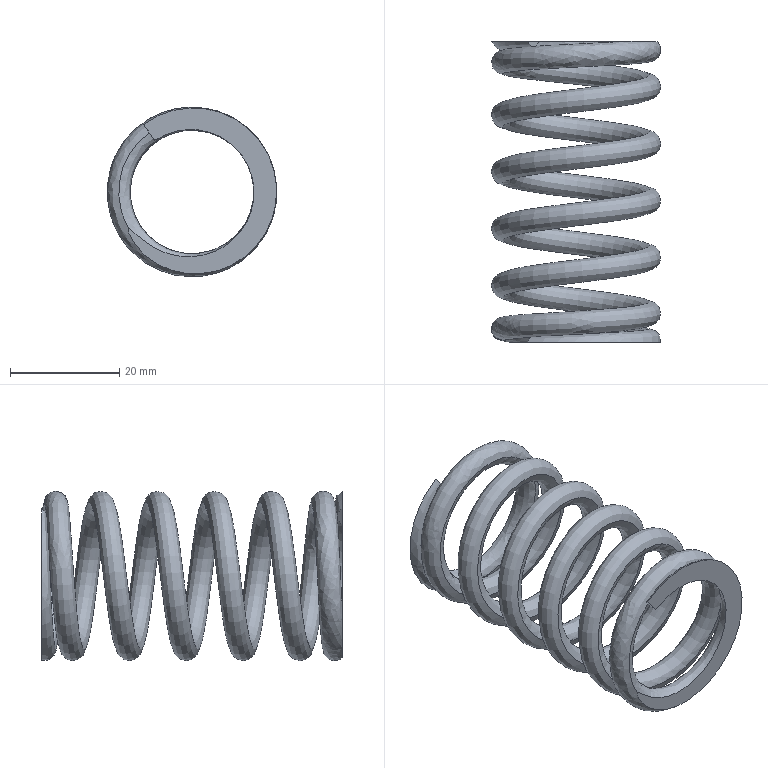Part | SolidWorks | features BaseBody 1 | 1 solid | 6 faces | box 31 x 55 x 31.002 mm | volume 7525 mm3 | plane 4 | spline 2